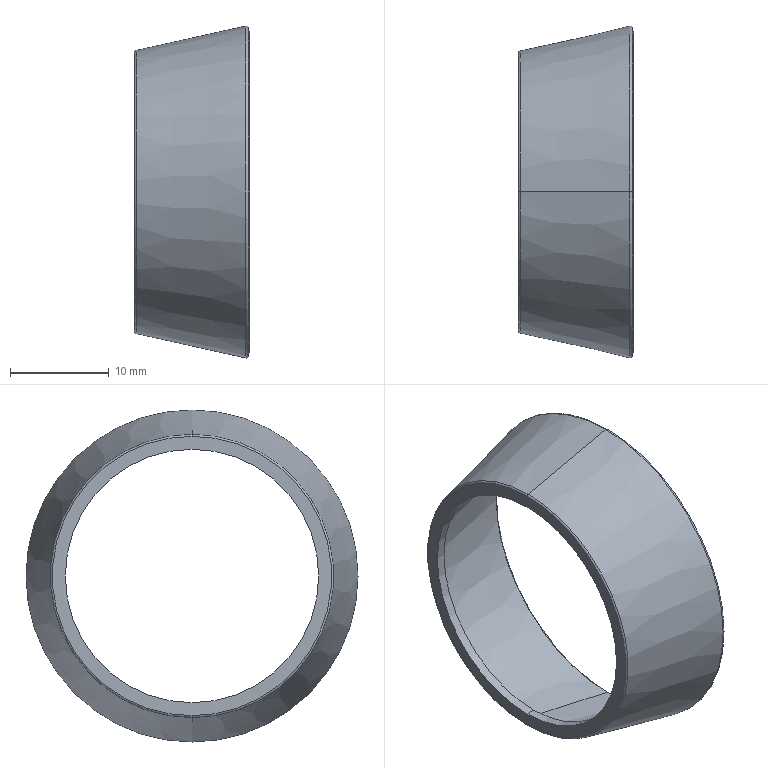Part | NX | features BREP 1 | 1 solid | 16 faces | box 11.643 x 33.606 x 33.606 mm | volume 1109 mm3 | torus 6 | cone 6 | plane 2 | cylinder 2 | commonest cylinder face diameters 25.643 x2
STEP:
#1=CARTESIAN_POINT('',(10.27,0.,16.646));
#2=VERTEX_POINT('',#1);
#3=CARTESIAN_POINT('',(10.032,0.,16.798));
#4=VERTEX_POINT('',#3);
#5=CARTESIAN_POINT('',(10.075,0.,16.603));
#6=DIRECTION('',(0.,-1.,0.));
#7=DIRECTION('',(0.,0.,1.));
#8=AXIS2_PLACEMENT_3D('',#5,#6,#7);
#9=CIRCLE('',#8,0.2);
#10=EDGE_CURVE('',#2,#4,#9,.T.);
#11=ORIENTED_EDGE('',*,*,#10,.F.);
#12=CARTESIAN_POINT('',(10.27,0.,-16.646));
#13=VERTEX_POINT('',#12);
#14=CARTESIAN_POINT('',(10.27,0.,0.));
#15=DIRECTION('',(-1.,0.,0.));
#16=DIRECTION('',(0.,0.,1.));
#17=AXIS2_PLACEMENT_3D('',#14,#15,#16);
#18=CIRCLE('',#17,16.646);
#19=EDGE_CURVE('',#2,#13,#18,.T.);
#20=ORIENTED_EDGE('',*,*,#19,.T.);
#21=CARTESIAN_POINT('',(10.032,0.,-16.798));
#22=VERTEX_POINT('',#21);
#23=CARTESIAN_POINT('',(10.075,0.,-16.603));
#24=DIRECTION('',(0.,1.,0.));
#25=DIRECTION('',(0.9763,0.,-0.2164));
#26=AXIS2_PLACEMENT_3D('',#23,#24,#25);
#27=CIRCLE('',#26,0.2);
#28=EDGE_CURVE('',#13,#22,#27,.T.);
#29=ORIENTED_EDGE('',*,*,#28,.T.);
#30=CARTESIAN_POINT('',(10.032,0.,0.));
#31=DIRECTION('',(1.,0.,0.));
#32=DIRECTION('',(0.,0.,-1.));
#33=AXIS2_PLACEMENT_3D('',#30,#31,#32);
#34=CIRCLE('',#33,16.798);
#35=EDGE_CURVE('',#22,#4,#34,.T.);
#36=ORIENTED_EDGE('',*,*,#35,.T.);
#37=EDGE_LOOP('',(#11,#20,#29,#36));
#38=FACE_BOUND('',#37,.T.);
#39=CARTESIAN_POINT('',(10.075,0.,0.));
#40=DIRECTION('',(1.,0.,0.));
#41=DIRECTION('',(0.,0.,-1.));
#42=AXIS2_PLACEMENT_3D('',#39,#40,#41);
#43=TOROIDAL_SURFACE('',#42,16.603,0.2);
#44=ADVANCED_FACE('',(#38),#43,.T.);
#45=CARTESIAN_POINT('',(-1.093,0.,14.332));
#46=VERTEX_POINT('',#45);
#47=CARTESIAN_POINT('',(10.032,0.,16.798));
#48=DIRECTION('',(-0.9763,0.,-0.2164));
#49=VECTOR('',#48,1000.);
#50=LINE('',#47,#49);
#51=EDGE_CURVE('',#46,#4,#50,.F.);
#52=ORIENTED_EDGE('',*,*,#51,.T.);
#53=ORIENTED_EDGE('',*,*,#35,.F.);
#54=CARTESIAN_POINT('',(-1.093,0.,-14.332));
#55=VERTEX_POINT('',#54);
#56=CARTESIAN_POINT('',(10.032,0.,-16.798));
#57=DIRECTION('',(-0.9763,0.,0.2164));
#58=VECTOR('',#57,1000.);
#59=LINE('',#56,#58);
#60=EDGE_CURVE('',#55,#22,#59,.F.);
#61=ORIENTED_EDGE('',*,*,#60,.F.);
#62=CARTESIAN_POINT('',(-1.093,0.,0.));
#63=DIRECTION('',(-1.,0.,0.));
#64=DIRECTION('',(0.,0.,1.));
#65=AXIS2_PLACEMENT_3D('',#62,#63,#64);
#66=CIRCLE('',#65,14.332);
#67=EDGE_CURVE('',#46,#55,#66,.T.);
#68=ORIENTED_EDGE('',*,*,#67,.F.);
#69=EDGE_LOOP('',(#52,#53,#61,#68));
#70=FACE_BOUND('',#69,.T.);
#71=CARTESIAN_POINT('',(4.469,0.,0.));
#72=DIRECTION('',(1.,0.,0.));
#73=DIRECTION('',(0.,0.,-1.));
#74=AXIS2_PLACEMENT_3D('',#71,#72,#73);
#75=CONICAL_SURFACE('',#74,15.565,0.2182);
#76=ADVANCED_FACE('',(#70),#75,.T.);
#77=CARTESIAN_POINT('',(-1.25,0.,14.137));
#78=VERTEX_POINT('',#77);
#79=CARTESIAN_POINT('',(-1.05,0.,14.137));
#80=DIRECTION('',(0.,-1.,0.));
#81=DIRECTION('',(-0.2164,0.,0.9763));
#82=AXIS2_PLACEMENT_3D('',#79,#80,#81);
#83=CIRCLE('',#82,0.2);
#84=EDGE_CURVE('',#78,#46,#83,.F.);
#85=ORIENTED_EDGE('',*,*,#84,.T.);
#86=ORIENTED_EDGE('',*,*,#67,.T.);
#87=CARTESIAN_POINT('',(-1.25,0.,-14.137));
#88=VERTEX_POINT('',#87);
#89=CARTESIAN_POINT('',(-1.05,0.,-14.137));
#90=DIRECTION('',(0.,1.,0.));
#91=DIRECTION('',(-0.2164,0.,-0.9763));
#92=AXIS2_PLACEMENT_3D('',#89,#90,#91);
#93=CIRCLE('',#92,0.2);
#94=EDGE_CURVE('',#88,#55,#93,.F.);
#95=ORIENTED_EDGE('',*,*,#94,.F.);
#96=CARTESIAN_POINT('',(-1.25,0.,0.));
#97=DIRECTION('',(-1.,0.,0.));
#98=DIRECTION('',(0.,0.,1.));
#99=AXIS2_PLACEMENT_3D('',#96,#97,#98);
#100=CIRCLE('',#99,14.137);
#101=EDGE_CURVE('',#78,#88,#100,.T.);
#102=ORIENTED_EDGE('',*,*,#101,.F.);
#103=EDGE_LOOP('',(#85,#86,#95,#102));
#104=FACE_BOUND('',#103,.T.);
#105=CARTESIAN_POINT('',(-1.05,0.,0.));
#106=DIRECTION('',(1.,0.,0.));
#107=DIRECTION('',(0.,0.,-1.));
#108=AXIS2_PLACEMENT_3D('',#105,#106,#107);
#109=TOROIDAL_SURFACE('',#108,14.137,0.2);
#110=ADVANCED_FACE('',(#104),#109,.T.);
#111=ORIENTED_EDGE('',*,*,#101,.T.);
#112=CARTESIAN_POINT('',(-1.25,0.,0.));
#113=DIRECTION('',(-1.,0.,0.));
#114=DIRECTION('',(0.,0.,-1.));
#115=AXIS2_PLACEMENT_3D('',#112,#113,#114);
#116=CIRCLE('',#115,14.137);
#117=EDGE_CURVE('',#88,#78,#116,.T.);
#118=ORIENTED_EDGE('',*,*,#117,.T.);
#119=EDGE_LOOP('',(#111,#118));
#120=FACE_BOUND('',#119,.T.);
#121=CARTESIAN_POINT('',(-1.25,0.,12.821));
#122=VERTEX_POINT('',#121);
#123=CARTESIAN_POINT('',(-1.25,0.,-12.821));
#124=VERTEX_POINT('',#123);
#125=CARTESIAN_POINT('',(-1.25,0.,0.));
#126=DIRECTION('',(1.,0.,0.));
#127=DIRECTION('',(0.,0.,1.));
#128=AXIS2_PLACEMENT_3D('',#125,#126,#127);
#129=CIRCLE('',#128,12.821);
#130=EDGE_CURVE('',#122,#124,#129,.T.);
#131=ORIENTED_EDGE('',*,*,#130,.T.);
#132=CARTESIAN_POINT('',(-1.25,0.,0.));
#133=DIRECTION('',(1.,0.,0.));
#134=DIRECTION('',(0.,0.,-1.));
#135=AXIS2_PLACEMENT_3D('',#132,#133,#134);
#136=CIRCLE('',#135,12.821);
#137=EDGE_CURVE('',#124,#122,#136,.T.);
#138=ORIENTED_EDGE('',*,*,#137,.T.);
#139=EDGE_LOOP('',(#131,#138));
#140=FACE_BOUND('',#139,.T.);
#141=CARTESIAN_POINT('',(-1.25,12.821,0.));
#142=DIRECTION('',(1.,0.,0.));
#143=DIRECTION('',(0.,1.,0.));
#144=AXIS2_PLACEMENT_3D('',#141,#142,#143);
#145=PLANE('',#144);
#146=ADVANCED_FACE('',(#120,#140),#145,.F.);
#147=ORIENTED_EDGE('',*,*,#117,.F.);
#148=ORIENTED_EDGE('',*,*,#94,.T.);
#149=CARTESIAN_POINT('',(-1.093,0.,0.));
#150=DIRECTION('',(-1.,0.,0.));
#151=DIRECTION('',(0.,0.,-1.));
#152=AXIS2_PLACEMENT_3D('',#149,#150,#151);
#153=CIRCLE('',#152,14.332);
#154=EDGE_CURVE('',#55,#46,#153,.T.);
#155=ORIENTED_EDGE('',*,*,#154,.T.);
#156=ORIENTED_EDGE('',*,*,#84,.F.);
#157=EDGE_LOOP('',(#147,#148,#155,#156));
#158=FACE_BOUND('',#157,.T.);
#159=CARTESIAN_POINT('',(-1.05,0.,0.));
#160=DIRECTION('',(1.,0.,0.));
#161=DIRECTION('',(0.,0.,-1.));
#162=AXIS2_PLACEMENT_3D('',#159,#160,#161);
#163=TOROIDAL_SURFACE('',#162,14.137,0.2);
#164=ADVANCED_FACE('',(#158),#163,.T.);
#165=ORIENTED_EDGE('',*,*,#154,.F.);
#166=ORIENTED_EDGE('',*,*,#60,.T.);
#167=CARTESIAN_POINT('',(10.032,0.,0.));
#168=DIRECTION('',(1.,0.,0.));
#169=DIRECTION('',(0.,0.,1.));
#170=AXIS2_PLACEMENT_3D('',#167,#168,#169);
#171=CIRCLE('',#170,16.798);
#172=EDGE_CURVE('',#4,#22,#171,.T.);
#173=ORIENTED_EDGE('',*,*,#172,.F.);
#174=ORIENTED_EDGE('',*,*,#51,.F.);
#175=EDGE_LOOP('',(#165,#166,#173,#174));
#176=FACE_BOUND('',#175,.T.);
#177=CARTESIAN_POINT('',(4.469,0.,0.));
#178=DIRECTION('',(1.,0.,0.));
#179=DIRECTION('',(0.,0.,-1.));
#180=AXIS2_PLACEMENT_3D('',#177,#178,#179);
#181=CONICAL_SURFACE('',#180,15.565,0.2182);
#182=ADVANCED_FACE('',(#176),#181,.T.);
#183=ORIENTED_EDGE('',*,*,#10,.T.);
#184=ORIENTED_EDGE('',*,*,#172,.T.);
#185=ORIENTED_EDGE('',*,*,#28,.F.);
#186=CARTESIAN_POINT('',(10.27,0.,0.));
#187=DIRECTION('',(-1.,0.,0.));
#188=DIRECTION('',(0.,0.,-1.));
#189=AXIS2_PLACEMENT_3D('',#186,#187,#188);
#190=CIRCLE('',#189,16.646);
#191=EDGE_CURVE('',#13,#2,#190,.T.);
#192=ORIENTED_EDGE('',*,*,#191,.T.);
#193=EDGE_LOOP('',(#183,#184,#185,#192));
#194=FACE_BOUND('',#193,.T.);
#195=CARTESIAN_POINT('',(10.075,0.,0.));
#196=DIRECTION('',(1.,0.,0.));
#197=DIRECTION('',(0.,0.,-1.));
#198=AXIS2_PLACEMENT_3D('',#195,#196,#197);
#199=TOROIDAL_SURFACE('',#198,16.603,0.2);
#200=ADVANCED_FACE('',(#194),#199,.T.);
#201=CARTESIAN_POINT('',(10.388,0.,16.114));
#202=VERTEX_POINT('',#201);
#203=CARTESIAN_POINT('',(10.388,0.,-16.114));
#204=VERTEX_POINT('',#203);
#205=CARTESIAN_POINT('',(10.388,0.,0.));
#206=DIRECTION('',(1.,0.,0.));
#207=DIRECTION('',(0.,0.,1.));
#208=AXIS2_PLACEMENT_3D('',#205,#206,#207);
#209=CIRCLE('',#208,16.114);
#210=EDGE_CURVE('',#202,#204,#209,.T.);
#211=ORIENTED_EDGE('',*,*,#210,.F.);
#212=CARTESIAN_POINT('',(10.27,0.,16.646));
#213=DIRECTION('',(0.2164,0.,-0.9763));
#214=VECTOR('',#213,1000.);
#215=LINE('',#212,#214);
#216=EDGE_CURVE('',#202,#2,#215,.F.);
#217=ORIENTED_EDGE('',*,*,#216,.T.);
#218=ORIENTED_EDGE('',*,*,#191,.F.);
#219=CARTESIAN_POINT('',(10.27,0.,-16.646));
#220=DIRECTION('',(0.2164,0.,0.9763));
#221=VECTOR('',#220,1000.);
#222=LINE('',#219,#221);
#223=EDGE_CURVE('',#204,#13,#222,.F.);
#224=ORIENTED_EDGE('',*,*,#223,.F.);
#225=EDGE_LOOP('',(#211,#217,#218,#224));
#226=FACE_BOUND('',#225,.T.);
#227=CARTESIAN_POINT('',(10.329,0.,0.));
#228=DIRECTION('',(-1.,0.,0.));
#229=DIRECTION('',(0.,0.,1.));
#230=AXIS2_PLACEMENT_3D('',#227,#228,#229);
#231=CONICAL_SURFACE('',#230,16.38,1.353);
#232=ADVANCED_FACE('',(#226),#231,.T.);
#233=ORIENTED_EDGE('',*,*,#223,.T.);
#234=ORIENTED_EDGE('',*,*,#19,.F.);
#235=ORIENTED_EDGE('',*,*,#216,.F.);
#236=CARTESIAN_POINT('',(10.388,0.,0.));
#237=DIRECTION('',(1.,0.,0.));
#238=DIRECTION('',(0.,0.,-1.));
#239=AXIS2_PLACEMENT_3D('',#236,#237,#238);
#240=CIRCLE('',#239,16.114);
#241=EDGE_CURVE('',#204,#202,#240,.T.);
#242=ORIENTED_EDGE('',*,*,#241,.F.);
#243=EDGE_LOOP('',(#233,#234,#235,#242));
#244=FACE_BOUND('',#243,.T.);
#245=CARTESIAN_POINT('',(10.329,0.,0.));
#246=DIRECTION('',(-1.,0.,0.));
#247=DIRECTION('',(0.,0.,1.));
#248=AXIS2_PLACEMENT_3D('',#245,#246,#247);
#249=CONICAL_SURFACE('',#248,16.38,1.353);
#250=ADVANCED_FACE('',(#244),#249,.T.);
#251=CARTESIAN_POINT('',(10.236,0.,15.876));
#252=VERTEX_POINT('',#251);
#253=CARTESIAN_POINT('',(10.193,0.,16.071));
#254=DIRECTION('',(0.,-1.,0.));
#255=DIRECTION('',(0.2164,0.,-0.9763));
#256=AXIS2_PLACEMENT_3D('',#253,#254,#255);
#257=CIRCLE('',#256,0.2);
#258=EDGE_CURVE('',#202,#252,#257,.F.);
#259=ORIENTED_EDGE('',*,*,#258,.T.);
#260=CARTESIAN_POINT('',(10.236,0.,-15.876));
#261=VERTEX_POINT('',#260);
#262=CARTESIAN_POINT('',(10.236,0.,0.));
#263=DIRECTION('',(-1.,0.,0.));
#264=DIRECTION('',(0.,0.,1.));
#265=AXIS2_PLACEMENT_3D('',#262,#263,#264);
#266=CIRCLE('',#265,15.876);
#267=EDGE_CURVE('',#252,#261,#266,.T.);
#268=ORIENTED_EDGE('',*,*,#267,.T.);
#269=CARTESIAN_POINT('',(10.193,0.,-16.071));
#270=DIRECTION('',(0.,1.,0.));
#271=DIRECTION('',(0.2164,0.,0.9763));
#272=AXIS2_PLACEMENT_3D('',#269,#270,#271);
#273=CIRCLE('',#272,0.2);
#274=EDGE_CURVE('',#204,#261,#273,.F.);
#275=ORIENTED_EDGE('',*,*,#274,.F.);
#276=ORIENTED_EDGE('',*,*,#241,.T.);
#277=EDGE_LOOP('',(#259,#268,#275,#276));
#278=FACE_BOUND('',#277,.T.);
#279=CARTESIAN_POINT('',(10.193,0.,0.));
#280=DIRECTION('',(1.,0.,0.));
#281=DIRECTION('',(0.,0.,-1.));
#282=AXIS2_PLACEMENT_3D('',#279,#280,#281);
#283=TOROIDAL_SURFACE('',#282,16.071,0.2);
#284=ADVANCED_FACE('',(#278),#283,.T.);
#285=ORIENTED_EDGE('',*,*,#210,.T.);
#286=ORIENTED_EDGE('',*,*,#274,.T.);
#287=CARTESIAN_POINT('',(10.236,0.,0.));
#288=DIRECTION('',(-1.,0.,0.));
#289=DIRECTION('',(0.,0.,-1.));
#290=AXIS2_PLACEMENT_3D('',#287,#288,#289);
#291=CIRCLE('',#290,15.876);
#292=EDGE_CURVE('',#261,#252,#291,.T.);
#293=ORIENTED_EDGE('',*,*,#292,.T.);
#294=ORIENTED_EDGE('',*,*,#258,.F.);
#295=EDGE_LOOP('',(#285,#286,#293,#294));
#296=FACE_BOUND('',#295,.T.);
#297=CARTESIAN_POINT('',(10.193,0.,0.));
#298=DIRECTION('',(1.,0.,0.));
#299=DIRECTION('',(0.,0.,-1.));
#300=AXIS2_PLACEMENT_3D('',#297,#298,#299);
#301=TOROIDAL_SURFACE('',#300,16.071,0.2);
#302=ADVANCED_FACE('',(#296),#301,.T.);
#303=CARTESIAN_POINT('',(-0.305,0.,13.539));
#304=VERTEX_POINT('',#303);
#305=CARTESIAN_POINT('',(10.236,0.,15.876));
#306=DIRECTION('',(-0.9763,0.,-0.2164));
#307=VECTOR('',#306,1000.);
#308=LINE('',#305,#307);
#309=EDGE_CURVE('',#304,#252,#308,.F.);
#310=ORIENTED_EDGE('',*,*,#309,.T.);
#311=ORIENTED_EDGE('',*,*,#292,.F.);
#312=CARTESIAN_POINT('',(-0.305,0.,-13.539));
#313=VERTEX_POINT('',#312);
#314=CARTESIAN_POINT('',(10.236,0.,-15.876));
#315=DIRECTION('',(-0.9763,0.,0.2164));
#316=VECTOR('',#315,1000.);
#317=LINE('',#314,#316);
#318=EDGE_CURVE('',#313,#261,#317,.F.);
#319=ORIENTED_EDGE('',*,*,#318,.F.);
#320=CARTESIAN_POINT('',(-0.305,0.,0.));
#321=DIRECTION('',(1.,0.,0.));
#322=DIRECTION('',(0.,0.,1.));
#323=AXIS2_PLACEMENT_3D('',#320,#321,#322);
#324=CIRCLE('',#323,13.539);
#325=EDGE_CURVE('',#304,#313,#324,.T.);
#326=ORIENTED_EDGE('',*,*,#325,.F.);
#327=EDGE_LOOP('',(#310,#311,#319,#326));
#328=FACE_BOUND('',#327,.T.);
#329=CARTESIAN_POINT('',(4.966,0.,0.));
#330=DIRECTION('',(1.,0.,0.));
#331=DIRECTION('',(0.,0.,-1.));
#332=AXIS2_PLACEMENT_3D('',#329,#330,#331);
#333=CONICAL_SURFACE('',#332,14.707,0.2182);
#334=ADVANCED_FACE('',(#328),#333,.F.);
#335=CARTESIAN_POINT('',(-0.305,0.,0.));
#336=DIRECTION('',(1.,0.,0.));
#337=DIRECTION('',(0.,0.,-1.));
#338=AXIS2_PLACEMENT_3D('',#335,#336,#337);
#339=CIRCLE('',#338,13.539);
#340=EDGE_CURVE('',#313,#304,#339,.T.);
#341=ORIENTED_EDGE('',*,*,#340,.T.);
#342=ORIENTED_EDGE('',*,*,#325,.T.);
#343=EDGE_LOOP('',(#341,#342));
#344=FACE_BOUND('',#343,.T.);
#345=CARTESIAN_POINT('',(-0.305,0.,-12.821));
#346=VERTEX_POINT('',#345);
#347=CARTESIAN_POINT('',(-0.305,0.,12.821));
#348=VERTEX_POINT('',#347);
#349=CARTESIAN_POINT('',(-0.305,0.,0.));
#350=DIRECTION('',(-1.,0.,0.));
#351=DIRECTION('',(0.,0.,-1.));
#352=AXIS2_PLACEMENT_3D('',#349,#350,#351);
#353=CIRCLE('',#352,12.821);
#354=EDGE_CURVE('',#346,#348,#353,.T.);
#355=ORIENTED_EDGE('',*,*,#354,.T.);
#356=CARTESIAN_POINT('',(-0.305,0.,0.));
#357=DIRECTION('',(-1.,0.,0.));
#358=DIRECTION('',(0.,0.,1.));
#359=AXIS2_PLACEMENT_3D('',#356,#357,#358);
#360=CIRCLE('',#359,12.821);
#361=EDGE_CURVE('',#348,#346,#360,.T.);
#362=ORIENTED_EDGE('',*,*,#361,.T.);
#363=EDGE_LOOP('',(#355,#362));
#364=FACE_BOUND('',#363,.T.);
#365=CARTESIAN_POINT('',(-0.305,13.539,0.));
#366=DIRECTION('',(-1.,0.,0.));
#367=DIRECTION('',(0.,0.,1.));
#368=AXIS2_PLACEMENT_3D('',#365,#366,#367);
#369=PLANE('',#368);
#370=ADVANCED_FACE('',(#344,#364),#369,.F.);
#371=ORIENTED_EDGE('',*,*,#340,.F.);
#372=ORIENTED_EDGE('',*,*,#318,.T.);
#373=ORIENTED_EDGE('',*,*,#267,.F.);
#374=ORIENTED_EDGE('',*,*,#309,.F.);
#375=EDGE_LOOP('',(#371,#372,#373,#374));
#376=FACE_BOUND('',#375,.T.);
#377=CARTESIAN_POINT('',(4.966,0.,0.));
#378=DIRECTION('',(1.,0.,0.));
#379=DIRECTION('',(0.,0.,-1.));
#380=AXIS2_PLACEMENT_3D('',#377,#378,#379);
#381=CONICAL_SURFACE('',#380,14.707,0.2182);
#382=ADVANCED_FACE('',(#376),#381,.F.);
#383=ORIENTED_EDGE('',*,*,#361,.F.);
#384=CARTESIAN_POINT('',(-1.25,0.,12.821));
#385=DIRECTION('',(1.,0.,0.));
#386=VECTOR('',#385,1000.);
#387=LINE('',#384,#386);
#388=EDGE_CURVE('',#348,#122,#387,.F.);
#389=ORIENTED_EDGE('',*,*,#388,.T.);
#390=ORIENTED_EDGE('',*,*,#137,.F.);
#391=CARTESIAN_POINT('',(-1.25,0.,-12.821));
#392=DIRECTION('',(1.,0.,0.));
#393=VECTOR('',#392,1000.);
#394=LINE('',#391,#393);
#395=EDGE_CURVE('',#346,#124,#394,.F.);
#396=ORIENTED_EDGE('',*,*,#395,.F.);
#397=EDGE_LOOP('',(#383,#389,#390,#396));
#398=FACE_BOUND('',#397,.T.);
#399=CARTESIAN_POINT('',(0.,0.,0.));
#400=DIRECTION('',(-1.,0.,0.));
#401=DIRECTION('',(0.,0.,1.));
#402=AXIS2_PLACEMENT_3D('',#399,#400,#401);
#403=CYLINDRICAL_SURFACE('',#402,12.821);
#404=ADVANCED_FACE('',(#398),#403,.F.);
#405=ORIENTED_EDGE('',*,*,#395,.T.);
#406=ORIENTED_EDGE('',*,*,#130,.F.);
#407=ORIENTED_EDGE('',*,*,#388,.F.);
#408=ORIENTED_EDGE('',*,*,#354,.F.);
#409=EDGE_LOOP('',(#405,#406,#407,#408));
#410=FACE_BOUND('',#409,.T.);
#411=CARTESIAN_POINT('',(0.,0.,0.));
#412=DIRECTION('',(-1.,0.,0.));
#413=DIRECTION('',(0.,0.,1.));
#414=AXIS2_PLACEMENT_3D('',#411,#412,#413);
#415=CYLINDRICAL_SURFACE('',#414,12.821);
#416=ADVANCED_FACE('',(#410),#415,.F.);
#417=CLOSED_SHELL('',(#44,#76,#110,#146,#164,#182,#200,#232,#250,#284,#302,#334,#370,#382,#404,#416));
#418=MANIFOLD_SOLID_BREP('',#417);
#419=(LENGTH_UNIT()NAMED_UNIT(*)SI_UNIT(.MILLI.,.METRE.));
#420=UNCERTAINTY_MEASURE_WITH_UNIT(LENGTH_MEASURE(0.00001),#419,'','');
#421=(NAMED_UNIT(*)PLANE_ANGLE_UNIT()SI_UNIT($,.RADIAN.));
#422=(NAMED_UNIT(*)SI_UNIT($,.STERADIAN.)SOLID_ANGLE_UNIT());
#423=(GEOMETRIC_REPRESENTATION_CONTEXT(3)GLOBAL_UNCERTAINTY_ASSIGNED_CONTEXT((#420))GLOBAL_UNIT_ASSIGNED_CONTEXT((#419,#421,#422))REPRESENTATION_CONTEXT('',''));
#424=ADVANCED_BREP_SHAPE_REPRESENTATION('',(#418),#423);